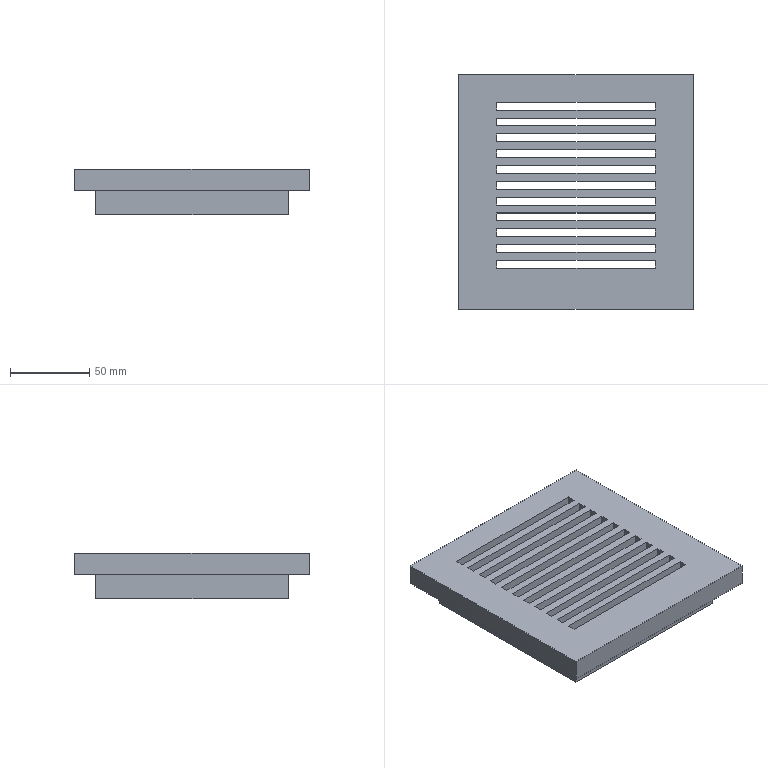Part | SolidWorks | features HoleWzd 2, ICE 2, Extrusion 1, LPattern 1 | 1 solid | 103 faces | box 148.5 x 148.5 x 29 mm | volume 366901 mm3 | plane 55 | cylinder 24 | cone 24 | commonest cylinder face diameters 5 x16 3.3 x8